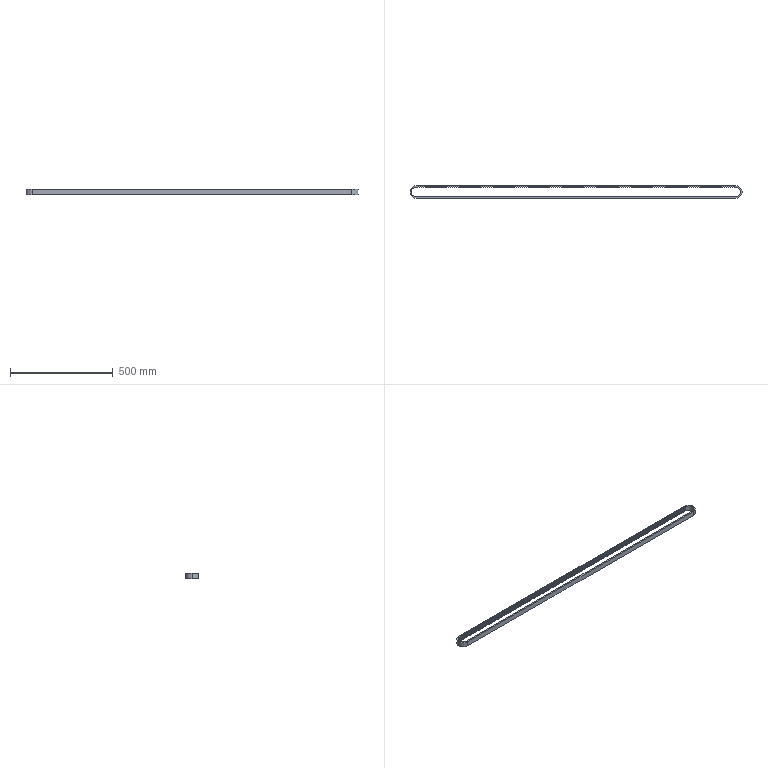Part | SolidWorks | features BaseBody 1 | 1 solid | 628 faces | box 1612 x 62 x 25 mm | volume 504931 mm3 | plane 622 | cylinder 6 | commonest cylinder face diameters 48 x3 62 x3